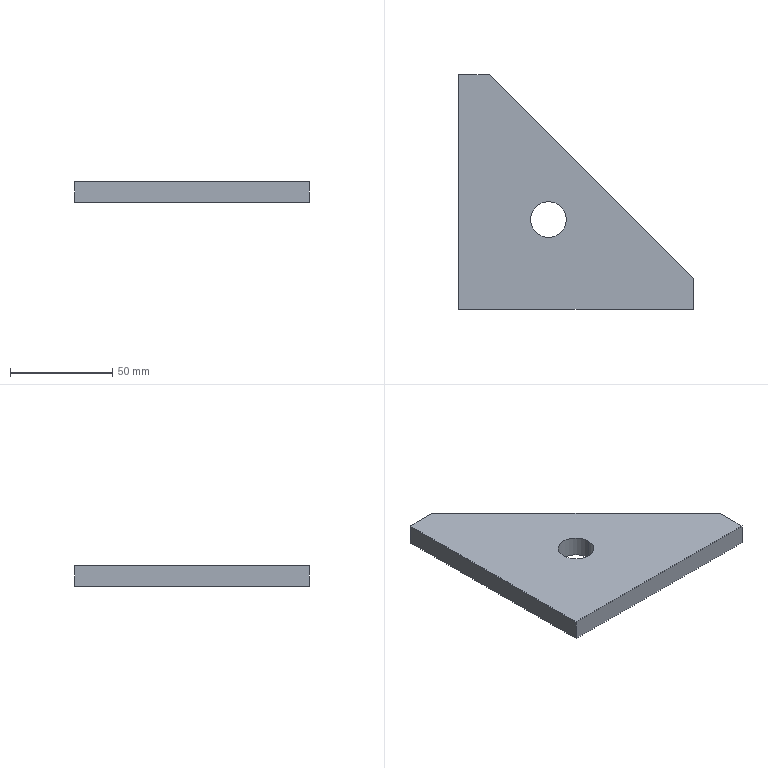Part | STEP file | PN_0001 Adjusting weld plate1 | 1 solid | 9 faces | box 115 x 115 x 10 mm | volume 79845 mm3 | plane 7 | cylinder 2 | commonest cylinder face diameters 17.5 x2
STEP:
#1=CARTESIAN_POINT('',(0.,0.,0.));
#2=DIRECTION('',(0.,0.,1.));
#3=DIRECTION('',(1.,0.,0.));
#4=AXIS2_PLACEMENT_3D('',#1,#2,#3);
#5=CARTESIAN_POINT('',(52.75,44.,0.));
#6=VERTEX_POINT('',#5);
#7=CARTESIAN_POINT('',(52.75,44.,10.));
#8=VERTEX_POINT('',#7);
#9=CARTESIAN_POINT('',(52.75,44.,10.));
#10=DIRECTION('',(0.,0.,1.));
#11=VECTOR('',#10,1.);
#12=LINE('',#9,#11);
#13=CARTESIAN_POINT('',(44.,44.,10.));
#14=DIRECTION('',(0.,0.,1.));
#15=DIRECTION('',(1.,0.,0.));
#16=AXIS2_PLACEMENT_3D('',#13,#14,#15);
#17=CYLINDRICAL_SURFACE('',#16,8.75);
#18=CARTESIAN_POINT('',(6.283,0.));
#19=DIRECTION('',(0.,1.));
#20=VECTOR('',#19,1.);
#21=LINE('',#18,#20);
#22=(GEOMETRIC_REPRESENTATION_CONTEXT(2)PARAMETRIC_REPRESENTATION_CONTEXT()REPRESENTATION_CONTEXT('',''));
#23=DEFINITIONAL_REPRESENTATION('',(#21),#22);
#24=PCURVE('',#17,#23);
#25=CARTESIAN_POINT('',(44.,44.,10.));
#26=DIRECTION('',(0.,0.,1.));
#27=DIRECTION('',(1.,0.,0.));
#28=AXIS2_PLACEMENT_3D('',#25,#26,#27);
#29=CYLINDRICAL_SURFACE('',#28,8.75);
#30=CARTESIAN_POINT('',(0.,0.));
#31=DIRECTION('',(0.,1.));
#32=VECTOR('',#31,1.);
#33=LINE('',#30,#32);
#34=(GEOMETRIC_REPRESENTATION_CONTEXT(2)PARAMETRIC_REPRESENTATION_CONTEXT()REPRESENTATION_CONTEXT('',''));
#35=DEFINITIONAL_REPRESENTATION('',(#33),#34);
#36=PCURVE('',#29,#35);
#37=SURFACE_CURVE('',#12,(#24,#36),.PCURVE_S1.);
#38=EDGE_CURVE('',#6,#8,#37,.T.);
#39=ORIENTED_EDGE('',*,*,#38,.T.);
#40=CARTESIAN_POINT('',(35.25,44.,10.));
#41=VERTEX_POINT('',#40);
#42=CARTESIAN_POINT('',(44.,44.,10.));
#43=DIRECTION('',(0.,0.,1.));
#44=DIRECTION('',(1.,0.,0.));
#45=AXIS2_PLACEMENT_3D('',#42,#43,#44);
#46=CIRCLE('',#45,8.75);
#47=CARTESIAN_POINT('',(0.,0.));
#48=DIRECTION('',(1.,0.));
#49=VECTOR('',#48,1.);
#50=LINE('',#47,#49);
#51=(GEOMETRIC_REPRESENTATION_CONTEXT(2)PARAMETRIC_REPRESENTATION_CONTEXT()REPRESENTATION_CONTEXT('',''));
#52=DEFINITIONAL_REPRESENTATION('',(#50),#51);
#53=PCURVE('',#17,#52);
#54=CARTESIAN_POINT('',(0.,0.,10.));
#55=DIRECTION('',(0.,0.,-1.));
#56=DIRECTION('',(-1.,0.,0.));
#57=AXIS2_PLACEMENT_3D('',#54,#55,#56);
#58=PLANE('',#57);
#59=CARTESIAN_POINT('',(-52.75,44.));
#60=CARTESIAN_POINT('',(-52.75,59.155));
#61=CARTESIAN_POINT('',(-39.625,51.578));
#62=CARTESIAN_POINT('',(-26.5,44.));
#63=CARTESIAN_POINT('',(-39.625,36.422));
#64=CARTESIAN_POINT('',(-52.75,28.845));
#65=CARTESIAN_POINT('',(-52.75,44.));
#66=(BOUNDED_CURVE()B_SPLINE_CURVE(2,(#59,#60,#61,#62,#63,#64,#65),.UNSPECIFIED.,.T.,.F.)B_SPLINE_CURVE_WITH_KNOTS((1,2,2,2,2,1),(-2.094,0.,2.094,4.189,6.283,8.378),.UNSPECIFIED.)CURVE()GEOMETRIC_REPRESENTATION_ITEM()RATIONAL_B_SPLINE_CURVE((1.,0.5,1.,0.5,1.,0.5,1.))REPRESENTATION_ITEM(''));
#67=(GEOMETRIC_REPRESENTATION_CONTEXT(2)PARAMETRIC_REPRESENTATION_CONTEXT()REPRESENTATION_CONTEXT('',''));
#68=DEFINITIONAL_REPRESENTATION('',(#66),#67);
#69=PCURVE('',#58,#68);
#70=SURFACE_CURVE('',#46,(#53,#69),.PCURVE_S1.);
#71=EDGE_CURVE('',#41,#8,#70,.T.);
#72=ORIENTED_EDGE('',*,*,#71,.F.);
#73=CARTESIAN_POINT('',(35.25,44.,0.));
#74=VERTEX_POINT('',#73);
#75=CARTESIAN_POINT('',(35.25,44.,10.));
#76=DIRECTION('',(0.,0.,1.));
#77=VECTOR('',#76,1.);
#78=LINE('',#75,#77);
#79=CARTESIAN_POINT('',(3.142,0.));
#80=DIRECTION('',(0.,1.));
#81=VECTOR('',#80,1.);
#82=LINE('',#79,#81);
#83=(GEOMETRIC_REPRESENTATION_CONTEXT(2)PARAMETRIC_REPRESENTATION_CONTEXT()REPRESENTATION_CONTEXT('',''));
#84=DEFINITIONAL_REPRESENTATION('',(#82),#83);
#85=PCURVE('',#17,#84);
#86=CARTESIAN_POINT('',(3.142,0.));
#87=DIRECTION('',(0.,1.));
#88=VECTOR('',#87,1.);
#89=LINE('',#86,#88);
#90=(GEOMETRIC_REPRESENTATION_CONTEXT(2)PARAMETRIC_REPRESENTATION_CONTEXT()REPRESENTATION_CONTEXT('',''));
#91=DEFINITIONAL_REPRESENTATION('',(#89),#90);
#92=PCURVE('',#29,#91);
#93=SURFACE_CURVE('',#78,(#85,#92),.PCURVE_S1.);
#94=EDGE_CURVE('',#74,#41,#93,.T.);
#95=ORIENTED_EDGE('',*,*,#94,.F.);
#96=CARTESIAN_POINT('',(44.,44.,0.));
#97=DIRECTION('',(0.,0.,-1.));
#98=DIRECTION('',(-1.,0.,0.));
#99=AXIS2_PLACEMENT_3D('',#96,#97,#98);
#100=CIRCLE('',#99,8.75);
#101=CARTESIAN_POINT('',(9.425,-10.));
#102=DIRECTION('',(-1.,0.));
#103=VECTOR('',#102,1.);
#104=LINE('',#101,#103);
#105=(GEOMETRIC_REPRESENTATION_CONTEXT(2)PARAMETRIC_REPRESENTATION_CONTEXT()REPRESENTATION_CONTEXT('',''));
#106=DEFINITIONAL_REPRESENTATION('',(#104),#105);
#107=PCURVE('',#17,#106);
#108=CARTESIAN_POINT('',(0.,0.,0.));
#109=DIRECTION('',(0.,0.,-1.));
#110=DIRECTION('',(-1.,0.,0.));
#111=AXIS2_PLACEMENT_3D('',#108,#109,#110);
#112=PLANE('',#111);
#113=CARTESIAN_POINT('',(-44.,44.));
#114=DIRECTION('',(1.,0.));
#115=AXIS2_PLACEMENT_2D('',#113,#114);
#116=CIRCLE('',#115,8.75);
#117=(GEOMETRIC_REPRESENTATION_CONTEXT(2)PARAMETRIC_REPRESENTATION_CONTEXT()REPRESENTATION_CONTEXT('',''));
#118=DEFINITIONAL_REPRESENTATION('',(#116),#117);
#119=PCURVE('',#112,#118);
#120=SURFACE_CURVE('',#100,(#107,#119),.PCURVE_S1.);
#121=EDGE_CURVE('',#6,#74,#120,.T.);
#122=ORIENTED_EDGE('',*,*,#121,.F.);
#123=EDGE_LOOP('',(#39,#72,#95,#122));
#124=FACE_BOUND('',#123,.F.);
#125=ADVANCED_FACE('',(#124),#17,.F.);
#126=CARTESIAN_POINT('',(0.,0.,0.));
#127=VERTEX_POINT('',#126);
#128=CARTESIAN_POINT('',(115.,0.,0.));
#129=VERTEX_POINT('',#128);
#130=CARTESIAN_POINT('',(130.,0.,0.));
#131=DIRECTION('',(1.,0.,0.));
#132=VECTOR('',#131,1.);
#133=LINE('',#130,#132);
#134=CARTESIAN_POINT('',(130.,0.,10.));
#135=DIRECTION('',(0.,1.,0.));
#136=DIRECTION('',(0.,0.,1.));
#137=AXIS2_PLACEMENT_3D('',#134,#135,#136);
#138=PLANE('',#137);
#139=CARTESIAN_POINT('',(-10.,0.));
#140=DIRECTION('',(0.,1.));
#141=VECTOR('',#140,1.);
#142=LINE('',#139,#141);
#143=(GEOMETRIC_REPRESENTATION_CONTEXT(2)PARAMETRIC_REPRESENTATION_CONTEXT()REPRESENTATION_CONTEXT('',''));
#144=DEFINITIONAL_REPRESENTATION('',(#142),#143);
#145=PCURVE('',#138,#144);
#146=CARTESIAN_POINT('',(-130.,0.));
#147=DIRECTION('',(-1.,0.));
#148=VECTOR('',#147,1.);
#149=LINE('',#146,#148);
#150=(GEOMETRIC_REPRESENTATION_CONTEXT(2)PARAMETRIC_REPRESENTATION_CONTEXT()REPRESENTATION_CONTEXT('',''));
#151=DEFINITIONAL_REPRESENTATION('',(#149),#150);
#152=PCURVE('',#112,#151);
#153=SURFACE_CURVE('',#133,(#145,#152),.PCURVE_S1.);
#154=EDGE_CURVE('',#127,#129,#153,.T.);
#155=ORIENTED_EDGE('',*,*,#154,.T.);
#156=CARTESIAN_POINT('',(115.,0.,10.));
#157=VERTEX_POINT('',#156);
#158=CARTESIAN_POINT('',(115.,0.,-0.001));
#159=DIRECTION('',(0.,0.,1.));
#160=VECTOR('',#159,1.);
#161=LINE('',#158,#160);
#162=CARTESIAN_POINT('',(-10.001,-15.));
#163=DIRECTION('',(1.,0.));
#164=VECTOR('',#163,1.);
#165=LINE('',#162,#164);
#166=(GEOMETRIC_REPRESENTATION_CONTEXT(2)PARAMETRIC_REPRESENTATION_CONTEXT()REPRESENTATION_CONTEXT('',''));
#167=DEFINITIONAL_REPRESENTATION('',(#165),#166);
#168=PCURVE('',#138,#167);
#169=CARTESIAN_POINT('',(115.,15.,-0.001));
#170=DIRECTION('',(-1.,0.,0.));
#171=DIRECTION('',(0.,0.,1.));
#172=AXIS2_PLACEMENT_3D('',#169,#170,#171);
#173=PLANE('',#172);
#174=CARTESIAN_POINT('',(0.,-15.));
#175=DIRECTION('',(1.,0.));
#176=VECTOR('',#175,1.);
#177=LINE('',#174,#176);
#178=(GEOMETRIC_REPRESENTATION_CONTEXT(2)PARAMETRIC_REPRESENTATION_CONTEXT()REPRESENTATION_CONTEXT('',''));
#179=DEFINITIONAL_REPRESENTATION('',(#177),#178);
#180=PCURVE('',#173,#179);
#181=SURFACE_CURVE('',#161,(#168,#180),.PCURVE_S1.);
#182=EDGE_CURVE('',#129,#157,#181,.T.);
#183=ORIENTED_EDGE('',*,*,#182,.T.);
#184=CARTESIAN_POINT('',(0.,0.,10.));
#185=VERTEX_POINT('',#184);
#186=CARTESIAN_POINT('',(130.,0.,10.));
#187=DIRECTION('',(1.,0.,0.));
#188=VECTOR('',#187,1.);
#189=LINE('',#186,#188);
#190=CARTESIAN_POINT('',(0.,0.));
#191=DIRECTION('',(0.,1.));
#192=VECTOR('',#191,1.);
#193=LINE('',#190,#192);
#194=(GEOMETRIC_REPRESENTATION_CONTEXT(2)PARAMETRIC_REPRESENTATION_CONTEXT()REPRESENTATION_CONTEXT('',''));
#195=DEFINITIONAL_REPRESENTATION('',(#193),#194);
#196=PCURVE('',#138,#195);
#197=CARTESIAN_POINT('',(-130.,0.));
#198=DIRECTION('',(-1.,0.));
#199=VECTOR('',#198,1.);
#200=LINE('',#197,#199);
#201=(GEOMETRIC_REPRESENTATION_CONTEXT(2)PARAMETRIC_REPRESENTATION_CONTEXT()REPRESENTATION_CONTEXT('',''));
#202=DEFINITIONAL_REPRESENTATION('',(#200),#201);
#203=PCURVE('',#58,#202);
#204=SURFACE_CURVE('',#189,(#196,#203),.PCURVE_S1.);
#205=EDGE_CURVE('',#185,#157,#204,.T.);
#206=ORIENTED_EDGE('',*,*,#205,.F.);
#207=CARTESIAN_POINT('',(0.,0.,10.));
#208=DIRECTION('',(0.,0.,-1.));
#209=VECTOR('',#208,1.);
#210=LINE('',#207,#209);
#211=CARTESIAN_POINT('',(0.,-130.));
#212=DIRECTION('',(-1.,0.));
#213=VECTOR('',#212,1.);
#214=LINE('',#211,#213);
#215=(GEOMETRIC_REPRESENTATION_CONTEXT(2)PARAMETRIC_REPRESENTATION_CONTEXT()REPRESENTATION_CONTEXT('',''));
#216=DEFINITIONAL_REPRESENTATION('',(#214),#215);
#217=PCURVE('',#138,#216);
#218=CARTESIAN_POINT('',(0.,0.,10.));
#219=DIRECTION('',(1.,0.,0.));
#220=DIRECTION('',(0.,1.,0.));
#221=AXIS2_PLACEMENT_3D('',#218,#219,#220);
#222=PLANE('',#221);
#223=CARTESIAN_POINT('',(0.,0.));
#224=DIRECTION('',(0.,-1.));
#225=VECTOR('',#224,1.);
#226=LINE('',#223,#225);
#227=(GEOMETRIC_REPRESENTATION_CONTEXT(2)PARAMETRIC_REPRESENTATION_CONTEXT()REPRESENTATION_CONTEXT('',''));
#228=DEFINITIONAL_REPRESENTATION('',(#226),#227);
#229=PCURVE('',#222,#228);
#230=SURFACE_CURVE('',#210,(#217,#229),.PCURVE_S1.);
#231=EDGE_CURVE('',#185,#127,#230,.T.);
#232=ORIENTED_EDGE('',*,*,#231,.T.);
#233=EDGE_LOOP('',(#155,#183,#206,#232));
#234=FACE_BOUND('',#233,.T.);
#235=ADVANCED_FACE('',(#234),#138,.F.);
#236=CARTESIAN_POINT('',(115.,15.,0.));
#237=VERTEX_POINT('',#236);
#238=CARTESIAN_POINT('',(15.,115.,0.));
#239=VERTEX_POINT('',#238);
#240=CARTESIAN_POINT('',(0.,130.,0.));
#241=DIRECTION('',(-0.7071,0.7071,0.));
#242=VECTOR('',#241,1.);
#243=LINE('',#240,#242);
#244=CARTESIAN_POINT('',(0.,130.,10.));
#245=DIRECTION('',(-0.7071,-0.7071,0.));
#246=DIRECTION('',(0.7071,-0.7071,0.));
#247=AXIS2_PLACEMENT_3D('',#244,#245,#246);
#248=PLANE('',#247);
#249=CARTESIAN_POINT('',(0.,-10.));
#250=DIRECTION('',(-1.,0.));
#251=VECTOR('',#250,1.);
#252=LINE('',#249,#251);
#253=(GEOMETRIC_REPRESENTATION_CONTEXT(2)PARAMETRIC_REPRESENTATION_CONTEXT()REPRESENTATION_CONTEXT('',''));
#254=DEFINITIONAL_REPRESENTATION('',(#252),#253);
#255=PCURVE('',#248,#254);
#256=CARTESIAN_POINT('',(0.,130.));
#257=DIRECTION('',(0.7071,0.7071));
#258=VECTOR('',#257,1.);
#259=LINE('',#256,#258);
#260=(GEOMETRIC_REPRESENTATION_CONTEXT(2)PARAMETRIC_REPRESENTATION_CONTEXT()REPRESENTATION_CONTEXT('',''));
#261=DEFINITIONAL_REPRESENTATION('',(#259),#260);
#262=PCURVE('',#112,#261);
#263=SURFACE_CURVE('',#243,(#255,#262),.PCURVE_S1.);
#264=EDGE_CURVE('',#237,#239,#263,.T.);
#265=ORIENTED_EDGE('',*,*,#264,.T.);
#266=CARTESIAN_POINT('',(15.,115.,10.));
#267=VERTEX_POINT('',#266);
#268=CARTESIAN_POINT('',(15.,115.,-0.001));
#269=DIRECTION('',(0.,0.,1.));
#270=VECTOR('',#269,1.);
#271=LINE('',#268,#270);
#272=CARTESIAN_POINT('',(21.213,-10.001));
#273=DIRECTION('',(0.,1.));
#274=VECTOR('',#273,1.);
#275=LINE('',#272,#274);
#276=(GEOMETRIC_REPRESENTATION_CONTEXT(2)PARAMETRIC_REPRESENTATION_CONTEXT()REPRESENTATION_CONTEXT('',''));
#277=DEFINITIONAL_REPRESENTATION('',(#275),#276);
#278=PCURVE('',#248,#277);
#279=CARTESIAN_POINT('',(0.,115.,-0.001));
#280=DIRECTION('',(0.,-1.,0.));
#281=DIRECTION('',(0.,0.,-1.));
#282=AXIS2_PLACEMENT_3D('',#279,#280,#281);
#283=PLANE('',#282);
#284=CARTESIAN_POINT('',(0.,15.));
#285=DIRECTION('',(-1.,0.));
#286=VECTOR('',#285,1.);
#287=LINE('',#284,#286);
#288=(GEOMETRIC_REPRESENTATION_CONTEXT(2)PARAMETRIC_REPRESENTATION_CONTEXT()REPRESENTATION_CONTEXT('',''));
#289=DEFINITIONAL_REPRESENTATION('',(#287),#288);
#290=PCURVE('',#283,#289);
#291=SURFACE_CURVE('',#271,(#278,#290),.PCURVE_S1.);
#292=EDGE_CURVE('',#239,#267,#291,.T.);
#293=ORIENTED_EDGE('',*,*,#292,.T.);
#294=CARTESIAN_POINT('',(115.,15.,10.));
#295=VERTEX_POINT('',#294);
#296=CARTESIAN_POINT('',(0.,130.,10.));
#297=DIRECTION('',(-0.7071,0.7071,0.));
#298=VECTOR('',#297,1.);
#299=LINE('',#296,#298);
#300=CARTESIAN_POINT('',(0.,0.));
#301=DIRECTION('',(-1.,0.));
#302=VECTOR('',#301,1.);
#303=LINE('',#300,#302);
#304=(GEOMETRIC_REPRESENTATION_CONTEXT(2)PARAMETRIC_REPRESENTATION_CONTEXT()REPRESENTATION_CONTEXT('',''));
#305=DEFINITIONAL_REPRESENTATION('',(#303),#304);
#306=PCURVE('',#248,#305);
#307=CARTESIAN_POINT('',(0.,130.));
#308=DIRECTION('',(0.7071,0.7071));
#309=VECTOR('',#308,1.);
#310=LINE('',#307,#309);
#311=(GEOMETRIC_REPRESENTATION_CONTEXT(2)PARAMETRIC_REPRESENTATION_CONTEXT()REPRESENTATION_CONTEXT('',''));
#312=DEFINITIONAL_REPRESENTATION('',(#310),#311);
#313=PCURVE('',#58,#312);
#314=SURFACE_CURVE('',#299,(#306,#313),.PCURVE_S1.);
#315=EDGE_CURVE('',#295,#267,#314,.T.);
#316=ORIENTED_EDGE('',*,*,#315,.F.);
#317=CARTESIAN_POINT('',(115.,15.,-0.001));
#318=DIRECTION('',(0.,0.,1.));
#319=VECTOR('',#318,1.);
#320=LINE('',#317,#319);
#321=CARTESIAN_POINT('',(162.635,-10.001));
#322=DIRECTION('',(0.,1.));
#323=VECTOR('',#322,1.);
#324=LINE('',#321,#323);
#325=(GEOMETRIC_REPRESENTATION_CONTEXT(2)PARAMETRIC_REPRESENTATION_CONTEXT()REPRESENTATION_CONTEXT('',''));
#326=DEFINITIONAL_REPRESENTATION('',(#324),#325);
#327=PCURVE('',#248,#326);
#328=CARTESIAN_POINT('',(0.,0.));
#329=DIRECTION('',(1.,0.));
#330=VECTOR('',#329,1.);
#331=LINE('',#328,#330);
#332=(GEOMETRIC_REPRESENTATION_CONTEXT(2)PARAMETRIC_REPRESENTATION_CONTEXT()REPRESENTATION_CONTEXT('',''));
#333=DEFINITIONAL_REPRESENTATION('',(#331),#332);
#334=PCURVE('',#173,#333);
#335=SURFACE_CURVE('',#320,(#327,#334),.PCURVE_S1.);
#336=EDGE_CURVE('',#237,#295,#335,.T.);
#337=ORIENTED_EDGE('',*,*,#336,.F.);
#338=EDGE_LOOP('',(#265,#293,#316,#337));
#339=FACE_BOUND('',#338,.T.);
#340=ADVANCED_FACE('',(#339),#248,.F.);
#341=CARTESIAN_POINT('',(0.,115.,10.));
#342=VERTEX_POINT('',#341);
#343=CARTESIAN_POINT('',(0.,0.,10.));
#344=DIRECTION('',(0.,-1.,0.));
#345=VECTOR('',#344,1.);
#346=LINE('',#343,#345);
#347=CARTESIAN_POINT('',(0.,0.));
#348=DIRECTION('',(-1.,0.));
#349=VECTOR('',#348,1.);
#350=LINE('',#347,#349);
#351=(GEOMETRIC_REPRESENTATION_CONTEXT(2)PARAMETRIC_REPRESENTATION_CONTEXT()REPRESENTATION_CONTEXT('',''));
#352=DEFINITIONAL_REPRESENTATION('',(#350),#351);
#353=PCURVE('',#222,#352);
#354=CARTESIAN_POINT('',(0.,0.));
#355=DIRECTION('',(0.,-1.));
#356=VECTOR('',#355,1.);
#357=LINE('',#354,#356);
#358=(GEOMETRIC_REPRESENTATION_CONTEXT(2)PARAMETRIC_REPRESENTATION_CONTEXT()REPRESENTATION_CONTEXT('',''));
#359=DEFINITIONAL_REPRESENTATION('',(#357),#358);
#360=PCURVE('',#58,#359);
#361=SURFACE_CURVE('',#346,(#353,#360),.PCURVE_S1.);
#362=EDGE_CURVE('',#342,#185,#361,.T.);
#363=ORIENTED_EDGE('',*,*,#362,.F.);
#364=CARTESIAN_POINT('',(0.,115.,0.));
#365=VERTEX_POINT('',#364);
#366=CARTESIAN_POINT('',(0.,115.,-0.001));
#367=DIRECTION('',(0.,0.,1.));
#368=VECTOR('',#367,1.);
#369=LINE('',#366,#368);
#370=CARTESIAN_POINT('',(115.,-10.001));
#371=DIRECTION('',(0.,1.));
#372=VECTOR('',#371,1.);
#373=LINE('',#370,#372);
#374=(GEOMETRIC_REPRESENTATION_CONTEXT(2)PARAMETRIC_REPRESENTATION_CONTEXT()REPRESENTATION_CONTEXT('',''));
#375=DEFINITIONAL_REPRESENTATION('',(#373),#374);
#376=PCURVE('',#222,#375);
#377=CARTESIAN_POINT('',(0.,0.));
#378=DIRECTION('',(-1.,0.));
#379=VECTOR('',#378,1.);
#380=LINE('',#377,#379);
#381=(GEOMETRIC_REPRESENTATION_CONTEXT(2)PARAMETRIC_REPRESENTATION_CONTEXT()REPRESENTATION_CONTEXT('',''));
#382=DEFINITIONAL_REPRESENTATION('',(#380),#381);
#383=PCURVE('',#283,#382);
#384=SURFACE_CURVE('',#369,(#376,#383),.PCURVE_S1.);
#385=EDGE_CURVE('',#365,#342,#384,.T.);
#386=ORIENTED_EDGE('',*,*,#385,.F.);
#387=CARTESIAN_POINT('',(0.,0.,0.));
#388=DIRECTION('',(0.,-1.,0.));
#389=VECTOR('',#388,1.);
#390=LINE('',#387,#389);
#391=CARTESIAN_POINT('',(0.,-10.));
#392=DIRECTION('',(-1.,0.));
#393=VECTOR('',#392,1.);
#394=LINE('',#391,#393);
#395=(GEOMETRIC_REPRESENTATION_CONTEXT(2)PARAMETRIC_REPRESENTATION_CONTEXT()REPRESENTATION_CONTEXT('',''));
#396=DEFINITIONAL_REPRESENTATION('',(#394),#395);
#397=PCURVE('',#222,#396);
#398=CARTESIAN_POINT('',(0.,0.));
#399=DIRECTION('',(0.,-1.));
#400=VECTOR('',#399,1.);
#401=LINE('',#398,#400);
#402=(GEOMETRIC_REPRESENTATION_CONTEXT(2)PARAMETRIC_REPRESENTATION_CONTEXT()REPRESENTATION_CONTEXT('',''));
#403=DEFINITIONAL_REPRESENTATION('',(#401),#402);
#404=PCURVE('',#112,#403);
#405=SURFACE_CURVE('',#390,(#397,#404),.PCURVE_S1.);
#406=EDGE_CURVE('',#365,#127,#405,.T.);
#407=ORIENTED_EDGE('',*,*,#406,.T.);
#408=ORIENTED_EDGE('',*,*,#231,.F.);
#409=EDGE_LOOP('',(#363,#386,#407,#408));
#410=FACE_BOUND('',#409,.T.);
#411=ADVANCED_FACE('',(#410),#222,.F.);
#412=CARTESIAN_POINT('',(44.,44.,10.));
#413=DIRECTION('',(0.,0.,1.));
#414=DIRECTION('',(1.,0.,0.));
#415=AXIS2_PLACEMENT_3D('',#412,#413,#414);
#416=CIRCLE('',#415,8.75);
#417=CARTESIAN_POINT('',(-52.75,44.));
#418=CARTESIAN_POINT('',(-52.75,59.155));
#419=CARTESIAN_POINT('',(-39.625,51.578));
#420=CARTESIAN_POINT('',(-26.5,44.));
#421=CARTESIAN_POINT('',(-39.625,36.422));
#422=CARTESIAN_POINT('',(-52.75,28.845));
#423=CARTESIAN_POINT('',(-52.75,44.));
#424=(BOUNDED_CURVE()B_SPLINE_CURVE(2,(#417,#418,#419,#420,#421,#422,#423),.UNSPECIFIED.,.T.,.F.)B_SPLINE_CURVE_WITH_KNOTS((1,2,2,2,2,1),(-2.094,0.,2.094,4.189,6.283,8.378),.UNSPECIFIED.)CURVE()GEOMETRIC_REPRESENTATION_ITEM()RATIONAL_B_SPLINE_CURVE((1.,0.5,1.,0.5,1.,0.5,1.))REPRESENTATION_ITEM(''));
#425=(GEOMETRIC_REPRESENTATION_CONTEXT(2)PARAMETRIC_REPRESENTATION_CONTEXT()REPRESENTATION_CONTEXT('',''));
#426=DEFINITIONAL_REPRESENTATION('',(#424),#425);
#427=PCURVE('',#58,#426);
#428=CARTESIAN_POINT('',(0.,0.));
#429=DIRECTION('',(1.,0.));
#430=VECTOR('',#429,1.);
#431=LINE('',#428,#430);
#432=(GEOMETRIC_REPRESENTATION_CONTEXT(2)PARAMETRIC_REPRESENTATION_CONTEXT()REPRESENTATION_CONTEXT('',''));
#433=DEFINITIONAL_REPRESENTATION('',(#431),#432);
#434=PCURVE('',#29,#433);
#435=SURFACE_CURVE('',#416,(#427,#434),.PCURVE_S1.);
#436=EDGE_CURVE('',#8,#41,#435,.T.);
#437=ORIENTED_EDGE('',*,*,#436,.F.);
#438=ORIENTED_EDGE('',*,*,#71,.F.);
#439=EDGE_LOOP('',(#437,#438));
#440=FACE_BOUND('',#439,.T.);
#441=ORIENTED_EDGE('',*,*,#315,.T.);
#442=CARTESIAN_POINT('',(0.,115.,10.));
#443=DIRECTION('',(1.,0.,0.));
#444=VECTOR('',#443,1.);
#445=LINE('',#442,#444);
#446=CARTESIAN_POINT('',(0.,115.));
#447=DIRECTION('',(-1.,0.));
#448=VECTOR('',#447,1.);
#449=LINE('',#446,#448);
#450=(GEOMETRIC_REPRESENTATION_CONTEXT(2)PARAMETRIC_REPRESENTATION_CONTEXT()REPRESENTATION_CONTEXT('',''));
#451=DEFINITIONAL_REPRESENTATION('',(#449),#450);
#452=PCURVE('',#58,#451);
#453=CARTESIAN_POINT('',(-10.001,0.));
#454=DIRECTION('',(0.,1.));
#455=VECTOR('',#454,1.);
#456=LINE('',#453,#455);
#457=(GEOMETRIC_REPRESENTATION_CONTEXT(2)PARAMETRIC_REPRESENTATION_CONTEXT()REPRESENTATION_CONTEXT('',''));
#458=DEFINITIONAL_REPRESENTATION('',(#456),#457);
#459=PCURVE('',#283,#458);
#460=SURFACE_CURVE('',#445,(#452,#459),.PCURVE_S1.);
#461=EDGE_CURVE('',#342,#267,#460,.T.);
#462=ORIENTED_EDGE('',*,*,#461,.F.);
#463=ORIENTED_EDGE('',*,*,#362,.T.);
#464=ORIENTED_EDGE('',*,*,#205,.T.);
#465=CARTESIAN_POINT('',(115.,15.,10.));
#466=DIRECTION('',(0.,-1.,0.));
#467=VECTOR('',#466,1.);
#468=LINE('',#465,#467);
#469=CARTESIAN_POINT('',(-115.,15.));
#470=DIRECTION('',(0.,-1.));
#471=VECTOR('',#470,1.);
#472=LINE('',#469,#471);
#473=(GEOMETRIC_REPRESENTATION_CONTEXT(2)PARAMETRIC_REPRESENTATION_CONTEXT()REPRESENTATION_CONTEXT('',''));
#474=DEFINITIONAL_REPRESENTATION('',(#472),#473);
#475=PCURVE('',#58,#474);
#476=CARTESIAN_POINT('',(10.001,0.));
#477=DIRECTION('',(0.,-1.));
#478=VECTOR('',#477,1.);
#479=LINE('',#476,#478);
#480=(GEOMETRIC_REPRESENTATION_CONTEXT(2)PARAMETRIC_REPRESENTATION_CONTEXT()REPRESENTATION_CONTEXT('',''));
#481=DEFINITIONAL_REPRESENTATION('',(#479),#480);
#482=PCURVE('',#173,#481);
#483=SURFACE_CURVE('',#468,(#475,#482),.PCURVE_S1.);
#484=EDGE_CURVE('',#295,#157,#483,.T.);
#485=ORIENTED_EDGE('',*,*,#484,.F.);
#486=EDGE_LOOP('',(#441,#462,#463,#464,#485));
#487=FACE_BOUND('',#486,.T.);
#488=ADVANCED_FACE('',(#440,#487),#58,.F.);
#489=CARTESIAN_POINT('',(0.,115.,0.));
#490=DIRECTION('',(1.,0.,0.));
#491=VECTOR('',#490,1.);
#492=LINE('',#489,#491);
#493=CARTESIAN_POINT('',(0.,115.));
#494=DIRECTION('',(-1.,0.));
#495=VECTOR('',#494,1.);
#496=LINE('',#493,#495);
#497=(GEOMETRIC_REPRESENTATION_CONTEXT(2)PARAMETRIC_REPRESENTATION_CONTEXT()REPRESENTATION_CONTEXT('',''));
#498=DEFINITIONAL_REPRESENTATION('',(#496),#497);
#499=PCURVE('',#112,#498);
#500=CARTESIAN_POINT('',(-0.001,0.));
#501=DIRECTION('',(0.,1.));
#502=VECTOR('',#501,1.);
#503=LINE('',#500,#502);
#504=(GEOMETRIC_REPRESENTATION_CONTEXT(2)PARAMETRIC_REPRESENTATION_CONTEXT()REPRESENTATION_CONTEXT('',''));
#505=DEFINITIONAL_REPRESENTATION('',(#503),#504);
#506=PCURVE('',#283,#505);
#507=SURFACE_CURVE('',#492,(#499,#506),.PCURVE_S1.);
#508=EDGE_CURVE('',#365,#239,#507,.T.);
#509=ORIENTED_EDGE('',*,*,#508,.T.);
#510=ORIENTED_EDGE('',*,*,#264,.F.);
#511=CARTESIAN_POINT('',(115.,15.,0.));
#512=DIRECTION('',(0.,-1.,0.));
#513=VECTOR('',#512,1.);
#514=LINE('',#511,#513);
#515=CARTESIAN_POINT('',(-115.,15.));
#516=DIRECTION('',(0.,-1.));
#517=VECTOR('',#516,1.);
#518=LINE('',#515,#517);
#519=(GEOMETRIC_REPRESENTATION_CONTEXT(2)PARAMETRIC_REPRESENTATION_CONTEXT()REPRESENTATION_CONTEXT('',''));
#520=DEFINITIONAL_REPRESENTATION('',(#518),#519);
#521=PCURVE('',#112,#520);
#522=CARTESIAN_POINT('',(0.001,0.));
#523=DIRECTION('',(0.,-1.));
#524=VECTOR('',#523,1.);
#525=LINE('',#522,#524);
#526=(GEOMETRIC_REPRESENTATION_CONTEXT(2)PARAMETRIC_REPRESENTATION_CONTEXT()REPRESENTATION_CONTEXT('',''));
#527=DEFINITIONAL_REPRESENTATION('',(#525),#526);
#528=PCURVE('',#173,#527);
#529=SURFACE_CURVE('',#514,(#521,#528),.PCURVE_S1.);
#530=EDGE_CURVE('',#237,#129,#529,.T.);
#531=ORIENTED_EDGE('',*,*,#530,.T.);
#532=ORIENTED_EDGE('',*,*,#154,.F.);
#533=ORIENTED_EDGE('',*,*,#406,.F.);
#534=EDGE_LOOP('',(#509,#510,#531,#532,#533));
#535=FACE_BOUND('',#534,.T.);
#536=ORIENTED_EDGE('',*,*,#121,.F.);
#537=CARTESIAN_POINT('',(44.,44.,0.));
#538=DIRECTION('',(0.,0.,-1.));
#539=DIRECTION('',(-1.,0.,0.));
#540=AXIS2_PLACEMENT_3D('',#537,#538,#539);
#541=CIRCLE('',#540,8.75);
#542=CARTESIAN_POINT('',(-44.,44.));
#543=DIRECTION('',(1.,0.));
#544=AXIS2_PLACEMENT_2D('',#542,#543);
#545=CIRCLE('',#544,8.75);
#546=(GEOMETRIC_REPRESENTATION_CONTEXT(2)PARAMETRIC_REPRESENTATION_CONTEXT()REPRESENTATION_CONTEXT('',''));
#547=DEFINITIONAL_REPRESENTATION('',(#545),#546);
#548=PCURVE('',#112,#547);
#549=CARTESIAN_POINT('',(3.142,-10.));
#550=DIRECTION('',(-1.,0.));
#551=VECTOR('',#550,1.);
#552=LINE('',#549,#551);
#553=(GEOMETRIC_REPRESENTATION_CONTEXT(2)PARAMETRIC_REPRESENTATION_CONTEXT()REPRESENTATION_CONTEXT('',''));
#554=DEFINITIONAL_REPRESENTATION('',(#552),#553);
#555=PCURVE('',#29,#554);
#556=SURFACE_CURVE('',#541,(#548,#555),.PCURVE_S1.);
#557=EDGE_CURVE('',#74,#6,#556,.T.);
#558=ORIENTED_EDGE('',*,*,#557,.F.);
#559=EDGE_LOOP('',(#536,#558));
#560=FACE_BOUND('',#559,.T.);
#561=ADVANCED_FACE('',(#535,#560),#112,.T.);
#562=ORIENTED_EDGE('',*,*,#436,.F.);
#563=ORIENTED_EDGE('',*,*,#38,.F.);
#564=ORIENTED_EDGE('',*,*,#557,.F.);
#565=ORIENTED_EDGE('',*,*,#94,.T.);
#566=EDGE_LOOP('',(#562,#563,#564,#565));
#567=FACE_BOUND('',#566,.F.);
#568=ADVANCED_FACE('',(#567),#29,.F.);
#569=ORIENTED_EDGE('',*,*,#336,.T.);
#570=ORIENTED_EDGE('',*,*,#484,.T.);
#571=ORIENTED_EDGE('',*,*,#182,.F.);
#572=ORIENTED_EDGE('',*,*,#530,.F.);
#573=EDGE_LOOP('',(#569,#570,#571,#572));
#574=FACE_BOUND('',#573,.T.);
#575=ADVANCED_FACE('',(#574),#173,.F.);
#576=ORIENTED_EDGE('',*,*,#385,.T.);
#577=ORIENTED_EDGE('',*,*,#461,.T.);
#578=ORIENTED_EDGE('',*,*,#292,.F.);
#579=ORIENTED_EDGE('',*,*,#508,.F.);
#580=EDGE_LOOP('',(#576,#577,#578,#579));
#581=FACE_BOUND('',#580,.T.);
#582=ADVANCED_FACE('',(#581),#283,.F.);
#583=CLOSED_SHELL('',(#125,#235,#340,#411,#488,#561,#568,#575,#582));
#584=MANIFOLD_SOLID_BREP('',#583);
#585=(LENGTH_UNIT()NAMED_UNIT(*)SI_UNIT(.MILLI.,.METRE.));
#586=UNCERTAINTY_MEASURE_WITH_UNIT(LENGTH_MEASURE(0.0000001),#585,'','');
#587=(NAMED_UNIT(*)PLANE_ANGLE_UNIT()SI_UNIT($,.RADIAN.));
#588=(NAMED_UNIT(*)SI_UNIT($,.STERADIAN.)SOLID_ANGLE_UNIT());
#589=(GEOMETRIC_REPRESENTATION_CONTEXT(3)GLOBAL_UNCERTAINTY_ASSIGNED_CONTEXT((#586))GLOBAL_UNIT_ASSIGNED_CONTEXT((#585,#587,#588))REPRESENTATION_CONTEXT('',''));
#590=ADVANCED_BREP_SHAPE_REPRESENTATION('',(#4,#584),#589);